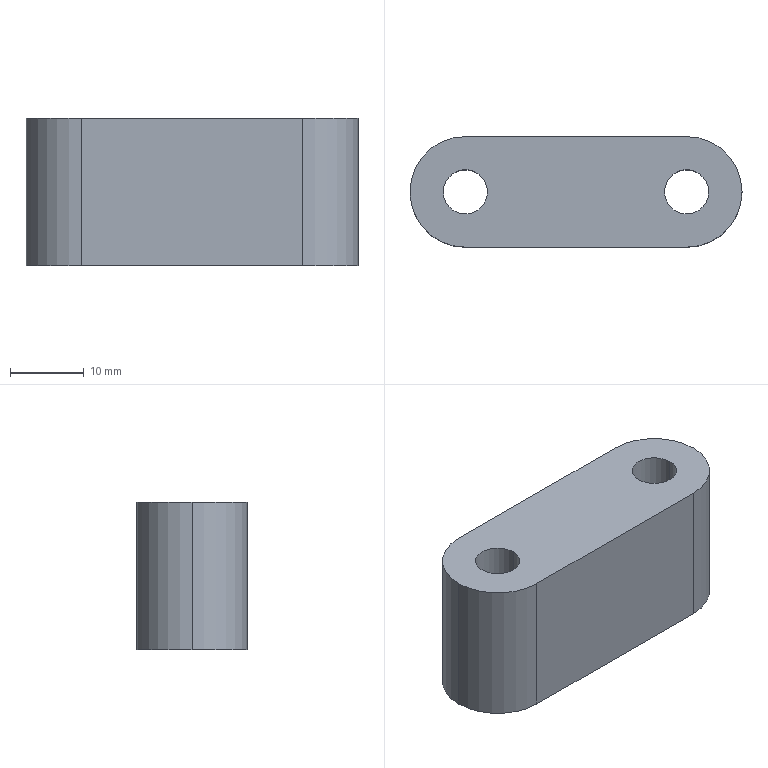Part | SolidWorks | features Extrusion 1 | 1 solid | 11 faces | box 45 x 15 x 20 mm | volume 11403 mm3 | cylinder 7 | plane 4 | commonest cylinder face diameters 6 x4 15 x3
STEP:
#1=CARTESIAN_POINT('',(27.,0.,20.));
#2=VERTEX_POINT('',#1);
#3=CARTESIAN_POINT('',(33.,0.,20.));
#4=VERTEX_POINT('',#3);
#5=CARTESIAN_POINT('',(30.,0.,20.));
#6=DIRECTION('',(0.,0.,1.));
#7=DIRECTION('',(1.,0.,0.));
#8=AXIS2_PLACEMENT_3D('',#5,#6,#7);
#9=CIRCLE('',#8,3.);
#10=EDGE_CURVE('',#2,#4,#9,.T.);
#11=ORIENTED_EDGE('',*,*,#10,.T.);
#12=CARTESIAN_POINT('',(33.,0.,0.));
#13=VERTEX_POINT('',#12);
#14=CARTESIAN_POINT('',(33.,0.,20.));
#15=DIRECTION('',(0.,0.,-1.));
#16=VECTOR('',#15,1000.);
#17=LINE('',#14,#16);
#18=EDGE_CURVE('',#4,#13,#17,.T.);
#19=ORIENTED_EDGE('',*,*,#18,.T.);
#20=CARTESIAN_POINT('',(27.,0.,0.));
#21=VERTEX_POINT('',#20);
#22=CARTESIAN_POINT('',(30.,0.,0.));
#23=DIRECTION('',(0.,0.,1.));
#24=DIRECTION('',(1.,0.,0.));
#25=AXIS2_PLACEMENT_3D('',#22,#23,#24);
#26=CIRCLE('',#25,3.);
#27=EDGE_CURVE('',#21,#13,#26,.T.);
#28=ORIENTED_EDGE('',*,*,#27,.F.);
#29=CARTESIAN_POINT('',(27.,0.,20.));
#30=DIRECTION('',(0.,0.,-1.));
#31=VECTOR('',#30,1000.);
#32=LINE('',#29,#31);
#33=EDGE_CURVE('',#2,#21,#32,.T.);
#34=ORIENTED_EDGE('',*,*,#33,.F.);
#35=EDGE_LOOP('',(#11,#19,#28,#34));
#36=FACE_OUTER_BOUND('',#35,.T.);
#37=CARTESIAN_POINT('',(30.,0.,20.));
#38=DIRECTION('',(0.,0.,-1.));
#39=DIRECTION('',(-1.,0.,0.));
#40=AXIS2_PLACEMENT_3D('',#37,#38,#39);
#41=CYLINDRICAL_SURFACE('',#40,3.);
#42=ADVANCED_FACE('',(#36),#41,.F.);
#43=CARTESIAN_POINT('',(-3.,0.,20.));
#44=VERTEX_POINT('',#43);
#45=CARTESIAN_POINT('',(3.,0.,20.));
#46=VERTEX_POINT('',#45);
#47=CARTESIAN_POINT('',(0.,0.,20.));
#48=DIRECTION('',(0.,0.,1.));
#49=DIRECTION('',(1.,0.,0.));
#50=AXIS2_PLACEMENT_3D('',#47,#48,#49);
#51=CIRCLE('',#50,3.);
#52=EDGE_CURVE('',#44,#46,#51,.T.);
#53=ORIENTED_EDGE('',*,*,#52,.T.);
#54=CARTESIAN_POINT('',(3.,0.,0.));
#55=VERTEX_POINT('',#54);
#56=CARTESIAN_POINT('',(3.,0.,20.));
#57=DIRECTION('',(0.,0.,-1.));
#58=VECTOR('',#57,1000.);
#59=LINE('',#56,#58);
#60=EDGE_CURVE('',#46,#55,#59,.T.);
#61=ORIENTED_EDGE('',*,*,#60,.T.);
#62=CARTESIAN_POINT('',(-3.,0.,0.));
#63=VERTEX_POINT('',#62);
#64=CARTESIAN_POINT('',(0.,0.,0.));
#65=DIRECTION('',(0.,0.,1.));
#66=DIRECTION('',(1.,0.,0.));
#67=AXIS2_PLACEMENT_3D('',#64,#65,#66);
#68=CIRCLE('',#67,3.);
#69=EDGE_CURVE('',#63,#55,#68,.T.);
#70=ORIENTED_EDGE('',*,*,#69,.F.);
#71=CARTESIAN_POINT('',(-3.,0.,20.));
#72=DIRECTION('',(0.,0.,-1.));
#73=VECTOR('',#72,1000.);
#74=LINE('',#71,#73);
#75=EDGE_CURVE('',#44,#63,#74,.T.);
#76=ORIENTED_EDGE('',*,*,#75,.F.);
#77=EDGE_LOOP('',(#53,#61,#70,#76));
#78=FACE_OUTER_BOUND('',#77,.T.);
#79=CARTESIAN_POINT('',(0.,0.,20.));
#80=DIRECTION('',(0.,0.,-1.));
#81=DIRECTION('',(-1.,0.,0.));
#82=AXIS2_PLACEMENT_3D('',#79,#80,#81);
#83=CYLINDRICAL_SURFACE('',#82,3.);
#84=ADVANCED_FACE('',(#78),#83,.F.);
#85=CARTESIAN_POINT('',(-7.5,0.,20.));
#86=VERTEX_POINT('',#85);
#87=CARTESIAN_POINT('',(0.,-7.5,20.));
#88=VERTEX_POINT('',#87);
#89=CARTESIAN_POINT('',(0.,0.,20.));
#90=DIRECTION('',(0.,0.,1.));
#91=DIRECTION('',(1.,0.,0.));
#92=AXIS2_PLACEMENT_3D('',#89,#90,#91);
#93=CIRCLE('',#92,7.5);
#94=EDGE_CURVE('',#86,#88,#93,.T.);
#95=ORIENTED_EDGE('',*,*,#94,.F.);
#96=CARTESIAN_POINT('',(-7.5,0.,0.));
#97=VERTEX_POINT('',#96);
#98=CARTESIAN_POINT('',(-7.5,0.,20.));
#99=DIRECTION('',(0.,0.,-1.));
#100=VECTOR('',#99,1000.);
#101=LINE('',#98,#100);
#102=EDGE_CURVE('',#86,#97,#101,.T.);
#103=ORIENTED_EDGE('',*,*,#102,.T.);
#104=CARTESIAN_POINT('',(0.,-7.5,0.));
#105=VERTEX_POINT('',#104);
#106=CARTESIAN_POINT('',(0.,0.,0.));
#107=DIRECTION('',(0.,0.,1.));
#108=DIRECTION('',(1.,0.,0.));
#109=AXIS2_PLACEMENT_3D('',#106,#107,#108);
#110=CIRCLE('',#109,7.5);
#111=EDGE_CURVE('',#97,#105,#110,.T.);
#112=ORIENTED_EDGE('',*,*,#111,.T.);
#113=CARTESIAN_POINT('',(0.,-7.5,20.));
#114=DIRECTION('',(0.,0.,-1.));
#115=VECTOR('',#114,1000.);
#116=LINE('',#113,#115);
#117=EDGE_CURVE('',#88,#105,#116,.T.);
#118=ORIENTED_EDGE('',*,*,#117,.F.);
#119=EDGE_LOOP('',(#95,#103,#112,#118));
#120=FACE_OUTER_BOUND('',#119,.T.);
#121=CARTESIAN_POINT('',(0.,0.,20.));
#122=DIRECTION('',(0.,0.,-1.));
#123=DIRECTION('',(-1.,0.,0.));
#124=AXIS2_PLACEMENT_3D('',#121,#122,#123);
#125=CYLINDRICAL_SURFACE('',#124,7.5);
#126=ADVANCED_FACE('',(#120),#125,.T.);
#127=ORIENTED_EDGE('',*,*,#52,.F.);
#128=CARTESIAN_POINT('',(0.,0.,20.));
#129=DIRECTION('',(0.,0.,1.));
#130=DIRECTION('',(1.,0.,0.));
#131=AXIS2_PLACEMENT_3D('',#128,#129,#130);
#132=CIRCLE('',#131,3.);
#133=EDGE_CURVE('',#46,#44,#132,.T.);
#134=ORIENTED_EDGE('',*,*,#133,.F.);
#135=EDGE_LOOP('',(#127,#134));
#136=FACE_BOUND('',#135,.T.);
#137=CARTESIAN_POINT('',(0.,7.5,20.));
#138=VERTEX_POINT('',#137);
#139=CARTESIAN_POINT('',(0.,0.,20.));
#140=DIRECTION('',(0.,0.,1.));
#141=DIRECTION('',(1.,0.,0.));
#142=AXIS2_PLACEMENT_3D('',#139,#140,#141);
#143=CIRCLE('',#142,7.5);
#144=EDGE_CURVE('',#138,#86,#143,.T.);
#145=ORIENTED_EDGE('',*,*,#144,.T.);
#146=ORIENTED_EDGE('',*,*,#94,.T.);
#147=CARTESIAN_POINT('',(30.,-7.5,20.));
#148=VERTEX_POINT('',#147);
#149=CARTESIAN_POINT('',(0.,-7.5,20.));
#150=DIRECTION('',(1.,0.,0.));
#151=VECTOR('',#150,1000.);
#152=LINE('',#149,#151);
#153=EDGE_CURVE('',#88,#148,#152,.T.);
#154=ORIENTED_EDGE('',*,*,#153,.T.);
#155=CARTESIAN_POINT('',(30.,7.5,20.));
#156=VERTEX_POINT('',#155);
#157=CARTESIAN_POINT('',(30.,0.,20.));
#158=DIRECTION('',(0.,0.,1.));
#159=DIRECTION('',(1.,0.,0.));
#160=AXIS2_PLACEMENT_3D('',#157,#158,#159);
#161=CIRCLE('',#160,7.5);
#162=EDGE_CURVE('',#148,#156,#161,.T.);
#163=ORIENTED_EDGE('',*,*,#162,.T.);
#164=CARTESIAN_POINT('',(0.,7.5,20.));
#165=DIRECTION('',(-1.,0.,0.));
#166=VECTOR('',#165,1000.);
#167=LINE('',#164,#166);
#168=EDGE_CURVE('',#156,#138,#167,.T.);
#169=ORIENTED_EDGE('',*,*,#168,.T.);
#170=EDGE_LOOP('',(#145,#146,#154,#163,#169));
#171=FACE_OUTER_BOUND('',#170,.T.);
#172=ORIENTED_EDGE('',*,*,#10,.F.);
#173=CARTESIAN_POINT('',(30.,0.,20.));
#174=DIRECTION('',(0.,0.,1.));
#175=DIRECTION('',(1.,0.,0.));
#176=AXIS2_PLACEMENT_3D('',#173,#174,#175);
#177=CIRCLE('',#176,3.);
#178=EDGE_CURVE('',#4,#2,#177,.T.);
#179=ORIENTED_EDGE('',*,*,#178,.F.);
#180=EDGE_LOOP('',(#172,#179));
#181=FACE_BOUND('',#180,.T.);
#182=CARTESIAN_POINT('',(0.,0.,20.));
#183=DIRECTION('',(0.,0.,1.));
#184=DIRECTION('',(1.,0.,0.));
#185=AXIS2_PLACEMENT_3D('',#182,#183,#184);
#186=PLANE('',#185);
#187=ADVANCED_FACE('',(#136,#171,#181),#186,.T.);
#188=CARTESIAN_POINT('',(0.,7.5,0.));
#189=VERTEX_POINT('',#188);
#190=CARTESIAN_POINT('',(0.,0.,0.));
#191=DIRECTION('',(0.,0.,1.));
#192=DIRECTION('',(1.,0.,0.));
#193=AXIS2_PLACEMENT_3D('',#190,#191,#192);
#194=CIRCLE('',#193,7.5);
#195=EDGE_CURVE('',#189,#97,#194,.T.);
#196=ORIENTED_EDGE('',*,*,#195,.F.);
#197=CARTESIAN_POINT('',(30.,7.5,0.));
#198=VERTEX_POINT('',#197);
#199=CARTESIAN_POINT('',(0.,7.5,0.));
#200=DIRECTION('',(-1.,0.,0.));
#201=VECTOR('',#200,1000.);
#202=LINE('',#199,#201);
#203=EDGE_CURVE('',#198,#189,#202,.T.);
#204=ORIENTED_EDGE('',*,*,#203,.F.);
#205=CARTESIAN_POINT('',(30.,-7.5,0.));
#206=VERTEX_POINT('',#205);
#207=CARTESIAN_POINT('',(30.,0.,0.));
#208=DIRECTION('',(0.,0.,1.));
#209=DIRECTION('',(1.,0.,0.));
#210=AXIS2_PLACEMENT_3D('',#207,#208,#209);
#211=CIRCLE('',#210,7.5);
#212=EDGE_CURVE('',#206,#198,#211,.T.);
#213=ORIENTED_EDGE('',*,*,#212,.F.);
#214=CARTESIAN_POINT('',(0.,-7.5,0.));
#215=DIRECTION('',(1.,0.,0.));
#216=VECTOR('',#215,1000.);
#217=LINE('',#214,#216);
#218=EDGE_CURVE('',#105,#206,#217,.T.);
#219=ORIENTED_EDGE('',*,*,#218,.F.);
#220=ORIENTED_EDGE('',*,*,#111,.F.);
#221=EDGE_LOOP('',(#196,#204,#213,#219,#220));
#222=FACE_OUTER_BOUND('',#221,.T.);
#223=ORIENTED_EDGE('',*,*,#69,.T.);
#224=CARTESIAN_POINT('',(0.,0.,0.));
#225=DIRECTION('',(0.,0.,1.));
#226=DIRECTION('',(1.,0.,0.));
#227=AXIS2_PLACEMENT_3D('',#224,#225,#226);
#228=CIRCLE('',#227,3.);
#229=EDGE_CURVE('',#55,#63,#228,.T.);
#230=ORIENTED_EDGE('',*,*,#229,.T.);
#231=EDGE_LOOP('',(#223,#230));
#232=FACE_BOUND('',#231,.T.);
#233=ORIENTED_EDGE('',*,*,#27,.T.);
#234=CARTESIAN_POINT('',(30.,0.,0.));
#235=DIRECTION('',(0.,0.,1.));
#236=DIRECTION('',(1.,0.,0.));
#237=AXIS2_PLACEMENT_3D('',#234,#235,#236);
#238=CIRCLE('',#237,3.);
#239=EDGE_CURVE('',#13,#21,#238,.T.);
#240=ORIENTED_EDGE('',*,*,#239,.T.);
#241=EDGE_LOOP('',(#233,#240));
#242=FACE_BOUND('',#241,.T.);
#243=CARTESIAN_POINT('',(0.,0.,0.));
#244=DIRECTION('',(0.,0.,1.));
#245=DIRECTION('',(1.,0.,0.));
#246=AXIS2_PLACEMENT_3D('',#243,#244,#245);
#247=PLANE('',#246);
#248=ADVANCED_FACE('',(#222,#232,#242),#247,.F.);
#249=ORIENTED_EDGE('',*,*,#102,.F.);
#250=ORIENTED_EDGE('',*,*,#144,.F.);
#251=CARTESIAN_POINT('',(0.,7.5,20.));
#252=DIRECTION('',(0.,0.,-1.));
#253=VECTOR('',#252,1000.);
#254=LINE('',#251,#253);
#255=EDGE_CURVE('',#138,#189,#254,.T.);
#256=ORIENTED_EDGE('',*,*,#255,.T.);
#257=ORIENTED_EDGE('',*,*,#195,.T.);
#258=EDGE_LOOP('',(#249,#250,#256,#257));
#259=FACE_OUTER_BOUND('',#258,.T.);
#260=CARTESIAN_POINT('',(0.,0.,20.));
#261=DIRECTION('',(0.,0.,-1.));
#262=DIRECTION('',(-1.,0.,0.));
#263=AXIS2_PLACEMENT_3D('',#260,#261,#262);
#264=CYLINDRICAL_SURFACE('',#263,7.5);
#265=ADVANCED_FACE('',(#259),#264,.T.);
#266=ORIENTED_EDGE('',*,*,#218,.T.);
#267=CARTESIAN_POINT('',(30.,-7.5,20.));
#268=DIRECTION('',(0.,0.,-1.));
#269=VECTOR('',#268,1000.);
#270=LINE('',#267,#269);
#271=EDGE_CURVE('',#148,#206,#270,.T.);
#272=ORIENTED_EDGE('',*,*,#271,.F.);
#273=ORIENTED_EDGE('',*,*,#153,.F.);
#274=ORIENTED_EDGE('',*,*,#117,.T.);
#275=EDGE_LOOP('',(#266,#272,#273,#274));
#276=FACE_OUTER_BOUND('',#275,.T.);
#277=CARTESIAN_POINT('',(0.,-7.5,20.));
#278=DIRECTION('',(0.,1.,0.));
#279=DIRECTION('',(0.,0.,1.));
#280=AXIS2_PLACEMENT_3D('',#277,#278,#279);
#281=PLANE('',#280);
#282=ADVANCED_FACE('',(#276),#281,.F.);
#283=ORIENTED_EDGE('',*,*,#212,.T.);
#284=CARTESIAN_POINT('',(30.,7.5,20.));
#285=DIRECTION('',(0.,0.,-1.));
#286=VECTOR('',#285,1000.);
#287=LINE('',#284,#286);
#288=EDGE_CURVE('',#156,#198,#287,.T.);
#289=ORIENTED_EDGE('',*,*,#288,.F.);
#290=ORIENTED_EDGE('',*,*,#162,.F.);
#291=ORIENTED_EDGE('',*,*,#271,.T.);
#292=EDGE_LOOP('',(#283,#289,#290,#291));
#293=FACE_OUTER_BOUND('',#292,.T.);
#294=CARTESIAN_POINT('',(30.,0.,20.));
#295=DIRECTION('',(0.,0.,-1.));
#296=DIRECTION('',(-1.,0.,0.));
#297=AXIS2_PLACEMENT_3D('',#294,#295,#296);
#298=CYLINDRICAL_SURFACE('',#297,7.5);
#299=ADVANCED_FACE('',(#293),#298,.T.);
#300=ORIENTED_EDGE('',*,*,#203,.T.);
#301=ORIENTED_EDGE('',*,*,#255,.F.);
#302=ORIENTED_EDGE('',*,*,#168,.F.);
#303=ORIENTED_EDGE('',*,*,#288,.T.);
#304=EDGE_LOOP('',(#300,#301,#302,#303));
#305=FACE_OUTER_BOUND('',#304,.T.);
#306=CARTESIAN_POINT('',(0.,7.5,20.));
#307=DIRECTION('',(0.,-1.,0.));
#308=DIRECTION('',(0.,0.,-1.));
#309=AXIS2_PLACEMENT_3D('',#306,#307,#308);
#310=PLANE('',#309);
#311=ADVANCED_FACE('',(#305),#310,.F.);
#312=ORIENTED_EDGE('',*,*,#60,.F.);
#313=ORIENTED_EDGE('',*,*,#133,.T.);
#314=ORIENTED_EDGE('',*,*,#75,.T.);
#315=ORIENTED_EDGE('',*,*,#229,.F.);
#316=EDGE_LOOP('',(#312,#313,#314,#315));
#317=FACE_OUTER_BOUND('',#316,.T.);
#318=CARTESIAN_POINT('',(0.,0.,20.));
#319=DIRECTION('',(0.,0.,-1.));
#320=DIRECTION('',(-1.,0.,0.));
#321=AXIS2_PLACEMENT_3D('',#318,#319,#320);
#322=CYLINDRICAL_SURFACE('',#321,3.);
#323=ADVANCED_FACE('',(#317),#322,.F.);
#324=ORIENTED_EDGE('',*,*,#18,.F.);
#325=ORIENTED_EDGE('',*,*,#178,.T.);
#326=ORIENTED_EDGE('',*,*,#33,.T.);
#327=ORIENTED_EDGE('',*,*,#239,.F.);
#328=EDGE_LOOP('',(#324,#325,#326,#327));
#329=FACE_OUTER_BOUND('',#328,.T.);
#330=CARTESIAN_POINT('',(30.,0.,20.));
#331=DIRECTION('',(0.,0.,-1.));
#332=DIRECTION('',(-1.,0.,0.));
#333=AXIS2_PLACEMENT_3D('',#330,#331,#332);
#334=CYLINDRICAL_SURFACE('',#333,3.);
#335=ADVANCED_FACE('',(#329),#334,.F.);
#336=CLOSED_SHELL('',(#42,#84,#126,#187,#248,#265,#282,#299,#311,#323,#335));
#337=MANIFOLD_SOLID_BREP('',#336);
#338=CARTESIAN_POINT('',(0.,0.,0.));
#339=DIRECTION('',(0.,0.,1.));
#340=DIRECTION('',(1.,0.,0.));
#341=AXIS2_PLACEMENT_3D('',#338,#339,#340);
#342=(LENGTH_UNIT()NAMED_UNIT(*)SI_UNIT(.MILLI.,.METRE.));
#343=UNCERTAINTY_MEASURE_WITH_UNIT(LENGTH_MEASURE(0.00001),#342,'','');
#344=(NAMED_UNIT(*)PLANE_ANGLE_UNIT()SI_UNIT($,.RADIAN.));
#345=(NAMED_UNIT(*)SI_UNIT($,.STERADIAN.)SOLID_ANGLE_UNIT());
#346=(GEOMETRIC_REPRESENTATION_CONTEXT(3)GLOBAL_UNCERTAINTY_ASSIGNED_CONTEXT((#343))GLOBAL_UNIT_ASSIGNED_CONTEXT((#342,#344,#345))REPRESENTATION_CONTEXT('',''));
#347=ADVANCED_BREP_SHAPE_REPRESENTATION('',(#337,#341),#346);